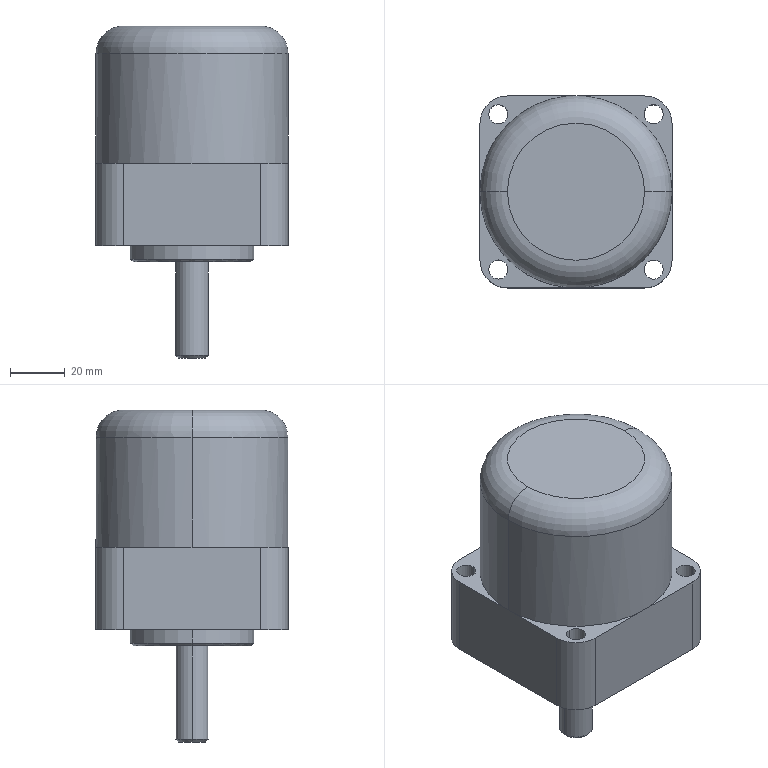Part | SolidWorks | features ICE 4, Chamfer 2, Fillet 2, CirPattern 1, Extrusion 1 | 1 solid | 36 faces | box 70 x 70 x 121 mm | volume 341225 mm3 | cylinder 18 | plane 12 | cone 4 | torus 2 | commonest cylinder face diameters 7 x8 20 x4 12 x2 45 x2 70 x2
STEP:
#1=CARTESIAN_POINT('',(-35.,0.,70.));
#2=VERTEX_POINT('',#1);
#3=CARTESIAN_POINT('',(35.,0.,70.));
#4=VERTEX_POINT('',#3);
#5=CARTESIAN_POINT('',(0.,0.,70.));
#6=DIRECTION('',(0.,0.,-1.));
#7=DIRECTION('',(1.,0.,0.));
#8=AXIS2_PLACEMENT_3D('',#5,#6,#7);
#9=CIRCLE('',#8,35.);
#10=EDGE_CURVE('',#2,#4,#9,.T.);
#11=ORIENTED_EDGE('',*,*,#10,.F.);
#12=CARTESIAN_POINT('',(-25.,0.,80.));
#13=VERTEX_POINT('',#12);
#14=CARTESIAN_POINT('',(-25.,0.,70.));
#15=DIRECTION('',(0.,1.,0.));
#16=DIRECTION('',(-1.,0.,0.));
#17=AXIS2_PLACEMENT_3D('',#14,#15,#16);
#18=CIRCLE('',#17,10.);
#19=EDGE_CURVE('',#2,#13,#18,.T.);
#20=ORIENTED_EDGE('',*,*,#19,.T.);
#21=CARTESIAN_POINT('',(25.,0.,80.));
#22=VERTEX_POINT('',#21);
#23=CARTESIAN_POINT('',(0.,0.,80.));
#24=DIRECTION('',(0.,0.,1.));
#25=DIRECTION('',(1.,0.,0.));
#26=AXIS2_PLACEMENT_3D('',#23,#24,#25);
#27=CIRCLE('',#26,25.);
#28=EDGE_CURVE('',#22,#13,#27,.T.);
#29=ORIENTED_EDGE('',*,*,#28,.F.);
#30=CARTESIAN_POINT('',(25.,0.,70.));
#31=DIRECTION('',(0.,-1.,0.));
#32=DIRECTION('',(0.,0.,-1.));
#33=AXIS2_PLACEMENT_3D('',#30,#31,#32);
#34=CIRCLE('',#33,10.);
#35=EDGE_CURVE('',#4,#22,#34,.T.);
#36=ORIENTED_EDGE('',*,*,#35,.F.);
#37=EDGE_LOOP('',(#11,#20,#29,#36));
#38=FACE_OUTER_BOUND('',#37,.T.);
#39=CARTESIAN_POINT('',(0.,0.,70.));
#40=DIRECTION('',(0.,0.,1.));
#41=DIRECTION('',(1.,0.,0.));
#42=AXIS2_PLACEMENT_3D('',#39,#40,#41);
#43=TOROIDAL_SURFACE('',#42,25.,10.);
#44=ADVANCED_FACE('',(#38),#43,.T.);
#45=ORIENTED_EDGE('',*,*,#10,.T.);
#46=CARTESIAN_POINT('',(35.,0.,30.));
#47=VERTEX_POINT('',#46);
#48=CARTESIAN_POINT('',(35.,0.,80.));
#49=DIRECTION('',(0.,0.,-1.));
#50=VECTOR('',#49,1000.);
#51=LINE('',#48,#50);
#52=EDGE_CURVE('',#4,#47,#51,.T.);
#53=ORIENTED_EDGE('',*,*,#52,.T.);
#54=CARTESIAN_POINT('',(0.,35.,30.));
#55=VERTEX_POINT('',#54);
#56=CARTESIAN_POINT('',(0.,0.,30.));
#57=DIRECTION('',(0.,0.,1.));
#58=DIRECTION('',(1.,0.,0.));
#59=AXIS2_PLACEMENT_3D('',#56,#57,#58);
#60=CIRCLE('',#59,35.);
#61=EDGE_CURVE('',#47,#55,#60,.T.);
#62=ORIENTED_EDGE('',*,*,#61,.T.);
#63=CARTESIAN_POINT('',(-35.,0.,30.));
#64=VERTEX_POINT('',#63);
#65=CARTESIAN_POINT('',(0.,0.,30.));
#66=DIRECTION('',(0.,0.,1.));
#67=DIRECTION('',(1.,0.,0.));
#68=AXIS2_PLACEMENT_3D('',#65,#66,#67);
#69=CIRCLE('',#68,35.);
#70=EDGE_CURVE('',#55,#64,#69,.T.);
#71=ORIENTED_EDGE('',*,*,#70,.T.);
#72=CARTESIAN_POINT('',(-35.,0.,80.));
#73=DIRECTION('',(0.,0.,-1.));
#74=VECTOR('',#73,1000.);
#75=LINE('',#72,#74);
#76=EDGE_CURVE('',#2,#64,#75,.T.);
#77=ORIENTED_EDGE('',*,*,#76,.F.);
#78=EDGE_LOOP('',(#45,#53,#62,#71,#77));
#79=FACE_OUTER_BOUND('',#78,.T.);
#80=CARTESIAN_POINT('',(0.,0.,80.));
#81=DIRECTION('',(0.,0.,-1.));
#82=DIRECTION('',(-1.,0.,0.));
#83=AXIS2_PLACEMENT_3D('',#80,#81,#82);
#84=CYLINDRICAL_SURFACE('',#83,35.);
#85=ADVANCED_FACE('',(#79),#84,.T.);
#86=CARTESIAN_POINT('',(28.284,31.784,0.));
#87=VERTEX_POINT('',#86);
#88=CARTESIAN_POINT('',(28.284,24.784,0.));
#89=VERTEX_POINT('',#88);
#90=CARTESIAN_POINT('',(28.284,28.284,0.));
#91=DIRECTION('',(0.,0.,1.));
#92=DIRECTION('',(0.,-1.,0.));
#93=AXIS2_PLACEMENT_3D('',#90,#91,#92);
#94=CIRCLE('',#93,3.5);
#95=EDGE_CURVE('',#87,#89,#94,.T.);
#96=ORIENTED_EDGE('',*,*,#95,.F.);
#97=CARTESIAN_POINT('',(28.284,31.784,30.));
#98=VERTEX_POINT('',#97);
#99=CARTESIAN_POINT('',(28.284,31.784,-30.));
#100=DIRECTION('',(0.,0.,1.));
#101=VECTOR('',#100,1000.);
#102=LINE('',#99,#101);
#103=EDGE_CURVE('',#87,#98,#102,.T.);
#104=ORIENTED_EDGE('',*,*,#103,.T.);
#105=CARTESIAN_POINT('',(28.284,24.784,30.));
#106=VERTEX_POINT('',#105);
#107=CARTESIAN_POINT('',(28.284,28.284,30.));
#108=DIRECTION('',(0.,0.,1.));
#109=DIRECTION('',(0.,-1.,0.));
#110=AXIS2_PLACEMENT_3D('',#107,#108,#109);
#111=CIRCLE('',#110,3.5);
#112=EDGE_CURVE('',#98,#106,#111,.T.);
#113=ORIENTED_EDGE('',*,*,#112,.T.);
#114=CARTESIAN_POINT('',(28.284,24.784,-30.));
#115=DIRECTION('',(0.,0.,1.));
#116=VECTOR('',#115,1000.);
#117=LINE('',#114,#116);
#118=EDGE_CURVE('',#89,#106,#117,.T.);
#119=ORIENTED_EDGE('',*,*,#118,.F.);
#120=EDGE_LOOP('',(#96,#104,#113,#119));
#121=FACE_OUTER_BOUND('',#120,.T.);
#122=CARTESIAN_POINT('',(28.284,28.284,-30.));
#123=DIRECTION('',(0.,0.,1.));
#124=DIRECTION('',(0.,-1.,0.));
#125=AXIS2_PLACEMENT_3D('',#122,#123,#124);
#126=CYLINDRICAL_SURFACE('',#125,3.5);
#127=ADVANCED_FACE('',(#121),#126,.F.);
#128=CARTESIAN_POINT('',(31.784,-28.284,0.));
#129=VERTEX_POINT('',#128);
#130=CARTESIAN_POINT('',(24.784,-28.284,0.));
#131=VERTEX_POINT('',#130);
#132=CARTESIAN_POINT('',(28.284,-28.284,0.));
#133=DIRECTION('',(0.,0.,1.));
#134=DIRECTION('',(-1.,0.,0.));
#135=AXIS2_PLACEMENT_3D('',#132,#133,#134);
#136=CIRCLE('',#135,3.5);
#137=EDGE_CURVE('',#129,#131,#136,.T.);
#138=ORIENTED_EDGE('',*,*,#137,.F.);
#139=CARTESIAN_POINT('',(31.784,-28.284,30.));
#140=VERTEX_POINT('',#139);
#141=CARTESIAN_POINT('',(31.784,-28.284,-30.));
#142=DIRECTION('',(0.,0.,1.));
#143=VECTOR('',#142,1000.);
#144=LINE('',#141,#143);
#145=EDGE_CURVE('',#129,#140,#144,.T.);
#146=ORIENTED_EDGE('',*,*,#145,.T.);
#147=CARTESIAN_POINT('',(24.784,-28.284,30.));
#148=VERTEX_POINT('',#147);
#149=CARTESIAN_POINT('',(28.284,-28.284,30.));
#150=DIRECTION('',(0.,0.,1.));
#151=DIRECTION('',(-1.,0.,0.));
#152=AXIS2_PLACEMENT_3D('',#149,#150,#151);
#153=CIRCLE('',#152,3.5);
#154=EDGE_CURVE('',#140,#148,#153,.T.);
#155=ORIENTED_EDGE('',*,*,#154,.T.);
#156=CARTESIAN_POINT('',(24.784,-28.284,-30.));
#157=DIRECTION('',(0.,0.,1.));
#158=VECTOR('',#157,1000.);
#159=LINE('',#156,#158);
#160=EDGE_CURVE('',#131,#148,#159,.T.);
#161=ORIENTED_EDGE('',*,*,#160,.F.);
#162=EDGE_LOOP('',(#138,#146,#155,#161));
#163=FACE_OUTER_BOUND('',#162,.T.);
#164=CARTESIAN_POINT('',(28.284,-28.284,-30.));
#165=DIRECTION('',(0.,0.,1.));
#166=DIRECTION('',(-1.,0.,0.));
#167=AXIS2_PLACEMENT_3D('',#164,#165,#166);
#168=CYLINDRICAL_SURFACE('',#167,3.5);
#169=ADVANCED_FACE('',(#163),#168,.F.);
#170=CARTESIAN_POINT('',(-28.284,-31.784,0.));
#171=VERTEX_POINT('',#170);
#172=CARTESIAN_POINT('',(-28.284,-24.784,0.));
#173=VERTEX_POINT('',#172);
#174=CARTESIAN_POINT('',(-28.284,-28.284,0.));
#175=DIRECTION('',(0.,0.,1.));
#176=DIRECTION('',(0.,1.,0.));
#177=AXIS2_PLACEMENT_3D('',#174,#175,#176);
#178=CIRCLE('',#177,3.5);
#179=EDGE_CURVE('',#171,#173,#178,.T.);
#180=ORIENTED_EDGE('',*,*,#179,.F.);
#181=CARTESIAN_POINT('',(-28.284,-31.784,30.));
#182=VERTEX_POINT('',#181);
#183=CARTESIAN_POINT('',(-28.284,-31.784,-30.));
#184=DIRECTION('',(0.,0.,1.));
#185=VECTOR('',#184,1000.);
#186=LINE('',#183,#185);
#187=EDGE_CURVE('',#171,#182,#186,.T.);
#188=ORIENTED_EDGE('',*,*,#187,.T.);
#189=CARTESIAN_POINT('',(-28.284,-24.784,30.));
#190=VERTEX_POINT('',#189);
#191=CARTESIAN_POINT('',(-28.284,-28.284,30.));
#192=DIRECTION('',(0.,0.,1.));
#193=DIRECTION('',(0.,1.,0.));
#194=AXIS2_PLACEMENT_3D('',#191,#192,#193);
#195=CIRCLE('',#194,3.5);
#196=EDGE_CURVE('',#182,#190,#195,.T.);
#197=ORIENTED_EDGE('',*,*,#196,.T.);
#198=CARTESIAN_POINT('',(-28.284,-24.784,-30.));
#199=DIRECTION('',(0.,0.,1.));
#200=VECTOR('',#199,1000.);
#201=LINE('',#198,#200);
#202=EDGE_CURVE('',#173,#190,#201,.T.);
#203=ORIENTED_EDGE('',*,*,#202,.F.);
#204=EDGE_LOOP('',(#180,#188,#197,#203));
#205=FACE_OUTER_BOUND('',#204,.T.);
#206=CARTESIAN_POINT('',(-28.284,-28.284,-30.));
#207=DIRECTION('',(0.,0.,1.));
#208=DIRECTION('',(0.,1.,0.));
#209=AXIS2_PLACEMENT_3D('',#206,#207,#208);
#210=CYLINDRICAL_SURFACE('',#209,3.5);
#211=ADVANCED_FACE('',(#205),#210,.F.);
#212=CARTESIAN_POINT('',(-21.5,0.,-6.));
#213=VERTEX_POINT('',#212);
#214=CARTESIAN_POINT('',(21.5,0.,-6.));
#215=VERTEX_POINT('',#214);
#216=CARTESIAN_POINT('',(0.,0.,-6.));
#217=DIRECTION('',(0.,0.,-1.));
#218=DIRECTION('',(-1.,0.,0.));
#219=AXIS2_PLACEMENT_3D('',#216,#217,#218);
#220=CIRCLE('',#219,21.5);
#221=EDGE_CURVE('',#213,#215,#220,.T.);
#222=ORIENTED_EDGE('',*,*,#221,.F.);
#223=CARTESIAN_POINT('',(-22.5,0.,-5.));
#224=VERTEX_POINT('',#223);
#225=CARTESIAN_POINT('',(-21.5,0.,-6.));
#226=DIRECTION('',(-0.7071,0.,0.7071));
#227=VECTOR('',#226,1000.);
#228=LINE('',#225,#227);
#229=EDGE_CURVE('',#213,#224,#228,.T.);
#230=ORIENTED_EDGE('',*,*,#229,.T.);
#231=CARTESIAN_POINT('',(22.5,0.,-5.));
#232=VERTEX_POINT('',#231);
#233=CARTESIAN_POINT('',(0.,0.,-5.));
#234=DIRECTION('',(0.,0.,1.));
#235=DIRECTION('',(-1.,0.,0.));
#236=AXIS2_PLACEMENT_3D('',#233,#234,#235);
#237=CIRCLE('',#236,22.5);
#238=EDGE_CURVE('',#232,#224,#237,.T.);
#239=ORIENTED_EDGE('',*,*,#238,.F.);
#240=CARTESIAN_POINT('',(21.5,0.,-6.));
#241=DIRECTION('',(0.7071,0.,0.7071));
#242=VECTOR('',#241,1000.);
#243=LINE('',#240,#242);
#244=EDGE_CURVE('',#215,#232,#243,.T.);
#245=ORIENTED_EDGE('',*,*,#244,.F.);
#246=EDGE_LOOP('',(#222,#230,#239,#245));
#247=FACE_OUTER_BOUND('',#246,.T.);
#248=CARTESIAN_POINT('',(0.,0.,-6.));
#249=DIRECTION('',(0.,0.,1.));
#250=DIRECTION('',(1.,0.,0.));
#251=AXIS2_PLACEMENT_3D('',#248,#249,#250);
#252=CONICAL_SURFACE('',#251,21.5,0.7854);
#253=ADVANCED_FACE('',(#247),#252,.T.);
#254=CARTESIAN_POINT('',(-5.,0.,-41.));
#255=VERTEX_POINT('',#254);
#256=CARTESIAN_POINT('',(5.,0.,-41.));
#257=VERTEX_POINT('',#256);
#258=CARTESIAN_POINT('',(0.,0.,-41.));
#259=DIRECTION('',(0.,0.,-1.));
#260=DIRECTION('',(-1.,0.,0.));
#261=AXIS2_PLACEMENT_3D('',#258,#259,#260);
#262=CIRCLE('',#261,5.);
#263=EDGE_CURVE('',#255,#257,#262,.T.);
#264=ORIENTED_EDGE('',*,*,#263,.F.);
#265=CARTESIAN_POINT('',(-6.,0.,-40.));
#266=VERTEX_POINT('',#265);
#267=CARTESIAN_POINT('',(-5.,0.,-41.));
#268=DIRECTION('',(-0.7071,0.,0.7071));
#269=VECTOR('',#268,1000.);
#270=LINE('',#267,#269);
#271=EDGE_CURVE('',#255,#266,#270,.T.);
#272=ORIENTED_EDGE('',*,*,#271,.T.);
#273=CARTESIAN_POINT('',(6.,0.,-40.));
#274=VERTEX_POINT('',#273);
#275=CARTESIAN_POINT('',(0.,0.,-40.));
#276=DIRECTION('',(0.,0.,1.));
#277=DIRECTION('',(-1.,0.,0.));
#278=AXIS2_PLACEMENT_3D('',#275,#276,#277);
#279=CIRCLE('',#278,6.);
#280=EDGE_CURVE('',#274,#266,#279,.T.);
#281=ORIENTED_EDGE('',*,*,#280,.F.);
#282=CARTESIAN_POINT('',(5.,0.,-41.));
#283=DIRECTION('',(0.7071,0.,0.7071));
#284=VECTOR('',#283,1000.);
#285=LINE('',#282,#284);
#286=EDGE_CURVE('',#257,#274,#285,.T.);
#287=ORIENTED_EDGE('',*,*,#286,.F.);
#288=EDGE_LOOP('',(#264,#272,#281,#287));
#289=FACE_OUTER_BOUND('',#288,.T.);
#290=CARTESIAN_POINT('',(0.,0.,-41.));
#291=DIRECTION('',(0.,0.,1.));
#292=DIRECTION('',(1.,0.,0.));
#293=AXIS2_PLACEMENT_3D('',#290,#291,#292);
#294=CONICAL_SURFACE('',#293,5.,0.7854);
#295=ADVANCED_FACE('',(#289),#294,.T.);
#296=ORIENTED_EDGE('',*,*,#280,.T.);
#297=CARTESIAN_POINT('',(-6.,0.,-6.));
#298=VERTEX_POINT('',#297);
#299=CARTESIAN_POINT('',(-6.,0.,-41.));
#300=DIRECTION('',(0.,0.,1.));
#301=VECTOR('',#300,1000.);
#302=LINE('',#299,#301);
#303=EDGE_CURVE('',#266,#298,#302,.T.);
#304=ORIENTED_EDGE('',*,*,#303,.T.);
#305=CARTESIAN_POINT('',(6.,0.,-6.));
#306=VERTEX_POINT('',#305);
#307=CARTESIAN_POINT('',(0.,0.,-6.));
#308=DIRECTION('',(0.,0.,-1.));
#309=DIRECTION('',(-1.,0.,0.));
#310=AXIS2_PLACEMENT_3D('',#307,#308,#309);
#311=CIRCLE('',#310,6.);
#312=EDGE_CURVE('',#298,#306,#311,.T.);
#313=ORIENTED_EDGE('',*,*,#312,.T.);
#314=CARTESIAN_POINT('',(6.,0.,-41.));
#315=DIRECTION('',(0.,0.,1.));
#316=VECTOR('',#315,1000.);
#317=LINE('',#314,#316);
#318=EDGE_CURVE('',#274,#306,#317,.T.);
#319=ORIENTED_EDGE('',*,*,#318,.F.);
#320=EDGE_LOOP('',(#296,#304,#313,#319));
#321=FACE_OUTER_BOUND('',#320,.T.);
#322=CARTESIAN_POINT('',(0.,0.,-41.));
#323=DIRECTION('',(0.,0.,1.));
#324=DIRECTION('',(1.,0.,0.));
#325=AXIS2_PLACEMENT_3D('',#322,#323,#324);
#326=CYLINDRICAL_SURFACE('',#325,6.);
#327=ADVANCED_FACE('',(#321),#326,.T.);
#328=ORIENTED_EDGE('',*,*,#238,.T.);
#329=CARTESIAN_POINT('',(-22.5,0.,0.));
#330=VERTEX_POINT('',#329);
#331=CARTESIAN_POINT('',(-22.5,0.,-6.));
#332=DIRECTION('',(0.,0.,1.));
#333=VECTOR('',#332,1000.);
#334=LINE('',#331,#333);
#335=EDGE_CURVE('',#224,#330,#334,.T.);
#336=ORIENTED_EDGE('',*,*,#335,.T.);
#337=CARTESIAN_POINT('',(22.5,0.,0.));
#338=VERTEX_POINT('',#337);
#339=CARTESIAN_POINT('',(0.,0.,0.));
#340=DIRECTION('',(0.,0.,-1.));
#341=DIRECTION('',(1.,0.,0.));
#342=AXIS2_PLACEMENT_3D('',#339,#340,#341);
#343=CIRCLE('',#342,22.5);
#344=EDGE_CURVE('',#330,#338,#343,.T.);
#345=ORIENTED_EDGE('',*,*,#344,.T.);
#346=CARTESIAN_POINT('',(22.5,0.,-6.));
#347=DIRECTION('',(0.,0.,1.));
#348=VECTOR('',#347,1000.);
#349=LINE('',#346,#348);
#350=EDGE_CURVE('',#232,#338,#349,.T.);
#351=ORIENTED_EDGE('',*,*,#350,.F.);
#352=EDGE_LOOP('',(#328,#336,#345,#351));
#353=FACE_OUTER_BOUND('',#352,.T.);
#354=CARTESIAN_POINT('',(0.,0.,-6.));
#355=DIRECTION('',(0.,0.,1.));
#356=DIRECTION('',(1.,0.,0.));
#357=AXIS2_PLACEMENT_3D('',#354,#355,#356);
#358=CYLINDRICAL_SURFACE('',#357,22.5);
#359=ADVANCED_FACE('',(#353),#358,.T.);
#360=CARTESIAN_POINT('',(-31.784,28.284,0.));
#361=VERTEX_POINT('',#360);
#362=CARTESIAN_POINT('',(-24.784,28.284,0.));
#363=VERTEX_POINT('',#362);
#364=CARTESIAN_POINT('',(-28.284,28.284,0.));
#365=DIRECTION('',(0.,0.,1.));
#366=DIRECTION('',(1.,0.,0.));
#367=AXIS2_PLACEMENT_3D('',#364,#365,#366);
#368=CIRCLE('',#367,3.5);
#369=EDGE_CURVE('',#361,#363,#368,.T.);
#370=ORIENTED_EDGE('',*,*,#369,.F.);
#371=CARTESIAN_POINT('',(-31.784,28.284,30.));
#372=VERTEX_POINT('',#371);
#373=CARTESIAN_POINT('',(-31.784,28.284,-30.));
#374=DIRECTION('',(0.,0.,1.));
#375=VECTOR('',#374,1000.);
#376=LINE('',#373,#375);
#377=EDGE_CURVE('',#361,#372,#376,.T.);
#378=ORIENTED_EDGE('',*,*,#377,.T.);
#379=CARTESIAN_POINT('',(-24.784,28.284,30.));
#380=VERTEX_POINT('',#379);
#381=CARTESIAN_POINT('',(-28.284,28.284,30.));
#382=DIRECTION('',(0.,0.,1.));
#383=DIRECTION('',(1.,0.,0.));
#384=AXIS2_PLACEMENT_3D('',#381,#382,#383);
#385=CIRCLE('',#384,3.5);
#386=EDGE_CURVE('',#372,#380,#385,.T.);
#387=ORIENTED_EDGE('',*,*,#386,.T.);
#388=CARTESIAN_POINT('',(-24.784,28.284,-30.));
#389=DIRECTION('',(0.,0.,1.));
#390=VECTOR('',#389,1000.);
#391=LINE('',#388,#390);
#392=EDGE_CURVE('',#363,#380,#391,.T.);
#393=ORIENTED_EDGE('',*,*,#392,.F.);
#394=EDGE_LOOP('',(#370,#378,#387,#393));
#395=FACE_OUTER_BOUND('',#394,.T.);
#396=CARTESIAN_POINT('',(-28.284,28.284,-30.));
#397=DIRECTION('',(0.,0.,1.));
#398=DIRECTION('',(1.,0.,0.));
#399=AXIS2_PLACEMENT_3D('',#396,#397,#398);
#400=CYLINDRICAL_SURFACE('',#399,3.5);
#401=ADVANCED_FACE('',(#395),#400,.F.);
#402=ORIENTED_EDGE('',*,*,#61,.F.);
#403=CARTESIAN_POINT('',(35.,25.,30.));
#404=VERTEX_POINT('',#403);
#405=CARTESIAN_POINT('',(35.,-35.,30.));
#406=DIRECTION('',(0.,1.,0.));
#407=VECTOR('',#406,1000.);
#408=LINE('',#405,#407);
#409=EDGE_CURVE('',#47,#404,#408,.T.);
#410=ORIENTED_EDGE('',*,*,#409,.T.);
#411=CARTESIAN_POINT('',(25.,35.,30.));
#412=VERTEX_POINT('',#411);
#413=CARTESIAN_POINT('',(25.,25.,30.));
#414=DIRECTION('',(0.,0.,1.));
#415=DIRECTION('',(1.,0.,0.));
#416=AXIS2_PLACEMENT_3D('',#413,#414,#415);
#417=CIRCLE('',#416,10.);
#418=EDGE_CURVE('',#404,#412,#417,.T.);
#419=ORIENTED_EDGE('',*,*,#418,.T.);
#420=CARTESIAN_POINT('',(35.,35.,30.));
#421=DIRECTION('',(-1.,0.,0.));
#422=VECTOR('',#421,1000.);
#423=LINE('',#420,#422);
#424=EDGE_CURVE('',#412,#55,#423,.T.);
#425=ORIENTED_EDGE('',*,*,#424,.T.);
#426=EDGE_LOOP('',(#402,#410,#419,#425));
#427=FACE_OUTER_BOUND('',#426,.T.);
#428=CARTESIAN_POINT('',(28.284,28.284,30.));
#429=DIRECTION('',(0.,0.,1.));
#430=DIRECTION('',(0.,-1.,0.));
#431=AXIS2_PLACEMENT_3D('',#428,#429,#430);
#432=CIRCLE('',#431,3.5);
#433=EDGE_CURVE('',#106,#98,#432,.T.);
#434=ORIENTED_EDGE('',*,*,#433,.F.);
#435=ORIENTED_EDGE('',*,*,#112,.F.);
#436=EDGE_LOOP('',(#434,#435));
#437=FACE_BOUND('',#436,.T.);
#438=CARTESIAN_POINT('',(0.,0.,30.));
#439=DIRECTION('',(0.,0.,1.));
#440=DIRECTION('',(1.,0.,0.));
#441=AXIS2_PLACEMENT_3D('',#438,#439,#440);
#442=PLANE('',#441);
#443=ADVANCED_FACE('',(#427,#437),#442,.T.);
#444=ORIENTED_EDGE('',*,*,#70,.F.);
#445=CARTESIAN_POINT('',(-25.,35.,30.));
#446=VERTEX_POINT('',#445);
#447=CARTESIAN_POINT('',(35.,35.,30.));
#448=DIRECTION('',(-1.,0.,0.));
#449=VECTOR('',#448,1000.);
#450=LINE('',#447,#449);
#451=EDGE_CURVE('',#55,#446,#450,.T.);
#452=ORIENTED_EDGE('',*,*,#451,.T.);
#453=CARTESIAN_POINT('',(-35.,25.,30.));
#454=VERTEX_POINT('',#453);
#455=CARTESIAN_POINT('',(-25.,25.,30.));
#456=DIRECTION('',(0.,0.,1.));
#457=DIRECTION('',(1.,0.,0.));
#458=AXIS2_PLACEMENT_3D('',#455,#456,#457);
#459=CIRCLE('',#458,10.);
#460=EDGE_CURVE('',#446,#454,#459,.T.);
#461=ORIENTED_EDGE('',*,*,#460,.T.);
#462=CARTESIAN_POINT('',(-35.,-35.,30.));
#463=DIRECTION('',(0.,-1.,0.));
#464=VECTOR('',#463,1000.);
#465=LINE('',#462,#464);
#466=EDGE_CURVE('',#454,#64,#465,.T.);
#467=ORIENTED_EDGE('',*,*,#466,.T.);
#468=EDGE_LOOP('',(#444,#452,#461,#467));
#469=FACE_OUTER_BOUND('',#468,.T.);
#470=CARTESIAN_POINT('',(-28.284,28.284,30.));
#471=DIRECTION('',(0.,0.,1.));
#472=DIRECTION('',(1.,0.,0.));
#473=AXIS2_PLACEMENT_3D('',#470,#471,#472);
#474=CIRCLE('',#473,3.5);
#475=EDGE_CURVE('',#380,#372,#474,.T.);
#476=ORIENTED_EDGE('',*,*,#475,.F.);
#477=ORIENTED_EDGE('',*,*,#386,.F.);
#478=EDGE_LOOP('',(#476,#477));
#479=FACE_BOUND('',#478,.T.);
#480=CARTESIAN_POINT('',(0.,0.,30.));
#481=DIRECTION('',(0.,0.,1.));
#482=DIRECTION('',(1.,0.,0.));
#483=AXIS2_PLACEMENT_3D('',#480,#481,#482);
#484=PLANE('',#483);
#485=ADVANCED_FACE('',(#469,#479),#484,.T.);
#486=CARTESIAN_POINT('',(0.,-35.,30.));
#487=VERTEX_POINT('',#486);
#488=CARTESIAN_POINT('',(0.,0.,30.));
#489=DIRECTION('',(0.,0.,1.));
#490=DIRECTION('',(1.,0.,0.));
#491=AXIS2_PLACEMENT_3D('',#488,#489,#490);
#492=CIRCLE('',#491,35.);
#493=EDGE_CURVE('',#64,#487,#492,.T.);
#494=ORIENTED_EDGE('',*,*,#493,.F.);
#495=CARTESIAN_POINT('',(-35.,-25.,30.));
#496=VERTEX_POINT('',#495);
#497=CARTESIAN_POINT('',(-35.,-35.,30.));
#498=DIRECTION('',(0.,-1.,0.));
#499=VECTOR('',#498,1000.);
#500=LINE('',#497,#499);
#501=EDGE_CURVE('',#64,#496,#500,.T.);
#502=ORIENTED_EDGE('',*,*,#501,.T.);
#503=CARTESIAN_POINT('',(-25.,-35.,30.));
#504=VERTEX_POINT('',#503);
#505=CARTESIAN_POINT('',(-25.,-25.,30.));
#506=DIRECTION('',(0.,0.,1.));
#507=DIRECTION('',(1.,0.,0.));
#508=AXIS2_PLACEMENT_3D('',#505,#506,#507);
#509=CIRCLE('',#508,10.);
#510=EDGE_CURVE('',#496,#504,#509,.T.);
#511=ORIENTED_EDGE('',*,*,#510,.T.);
#512=CARTESIAN_POINT('',(35.,-35.,30.));
#513=DIRECTION('',(1.,0.,0.));
#514=VECTOR('',#513,1000.);
#515=LINE('',#512,#514);
#516=EDGE_CURVE('',#504,#487,#515,.T.);
#517=ORIENTED_EDGE('',*,*,#516,.T.);
#518=EDGE_LOOP('',(#494,#502,#511,#517));
#519=FACE_OUTER_BOUND('',#518,.T.);
#520=CARTESIAN_POINT('',(-28.284,-28.284,30.));
#521=DIRECTION('',(0.,0.,1.));
#522=DIRECTION('',(0.,1.,0.));
#523=AXIS2_PLACEMENT_3D('',#520,#521,#522);
#524=CIRCLE('',#523,3.5);
#525=EDGE_CURVE('',#190,#182,#524,.T.);
#526=ORIENTED_EDGE('',*,*,#525,.F.);
#527=ORIENTED_EDGE('',*,*,#196,.F.);
#528=EDGE_LOOP('',(#526,#527));
#529=FACE_BOUND('',#528,.T.);
#530=CARTESIAN_POINT('',(0.,0.,30.));
#531=DIRECTION('',(0.,0.,1.));
#532=DIRECTION('',(1.,0.,0.));
#533=AXIS2_PLACEMENT_3D('',#530,#531,#532);
#534=PLANE('',#533);
#535=ADVANCED_FACE('',(#519,#529),#534,.T.);
#536=CARTESIAN_POINT('',(0.,0.,-6.));
#537=DIRECTION('',(0.,0.,-1.));
#538=DIRECTION('',(-1.,0.,0.));
#539=AXIS2_PLACEMENT_3D('',#536,#537,#538);
#540=CIRCLE('',#539,21.5);
#541=EDGE_CURVE('',#215,#213,#540,.T.);
#542=ORIENTED_EDGE('',*,*,#541,.T.);
#543=ORIENTED_EDGE('',*,*,#221,.T.);
#544=EDGE_LOOP('',(#542,#543));
#545=FACE_OUTER_BOUND('',#544,.T.);
#546=CARTESIAN_POINT('',(0.,0.,-6.));
#547=DIRECTION('',(0.,0.,-1.));
#548=DIRECTION('',(-1.,0.,0.));
#549=AXIS2_PLACEMENT_3D('',#546,#547,#548);
#550=CIRCLE('',#549,6.);
#551=EDGE_CURVE('',#306,#298,#550,.T.);
#552=ORIENTED_EDGE('',*,*,#551,.F.);
#553=ORIENTED_EDGE('',*,*,#312,.F.);
#554=EDGE_LOOP('',(#552,#553));
#555=FACE_BOUND('',#554,.T.);
#556=CARTESIAN_POINT('',(0.,0.,-6.));
#557=DIRECTION('',(0.,0.,-1.));
#558=DIRECTION('',(-1.,0.,0.));
#559=AXIS2_PLACEMENT_3D('',#556,#557,#558);
#560=PLANE('',#559);
#561=ADVANCED_FACE('',(#545,#555),#560,.T.);
#562=CARTESIAN_POINT('',(28.284,28.284,0.));
#563=DIRECTION('',(0.,0.,1.));
#564=DIRECTION('',(0.,-1.,0.));
#565=AXIS2_PLACEMENT_3D('',#562,#563,#564);
#566=CIRCLE('',#565,3.5);
#567=EDGE_CURVE('',#89,#87,#566,.T.);
#568=ORIENTED_EDGE('',*,*,#567,.T.);
#569=ORIENTED_EDGE('',*,*,#95,.T.);
#570=EDGE_LOOP('',(#568,#569));
#571=FACE_BOUND('',#570,.T.);
#572=CARTESIAN_POINT('',(28.284,-28.284,0.));
#573=DIRECTION('',(0.,0.,1.));
#574=DIRECTION('',(-1.,0.,0.));
#575=AXIS2_PLACEMENT_3D('',#572,#573,#574);
#576=CIRCLE('',#575,3.5);
#577=EDGE_CURVE('',#131,#129,#576,.T.);
#578=ORIENTED_EDGE('',*,*,#577,.T.);
#579=ORIENTED_EDGE('',*,*,#137,.T.);
#580=EDGE_LOOP('',(#578,#579));
#581=FACE_BOUND('',#580,.T.);
#582=CARTESIAN_POINT('',(-28.284,-28.284,0.));
#583=DIRECTION('',(0.,0.,1.));
#584=DIRECTION('',(0.,1.,0.));
#585=AXIS2_PLACEMENT_3D('',#582,#583,#584);
#586=CIRCLE('',#585,3.5);
#587=EDGE_CURVE('',#173,#171,#586,.T.);
#588=ORIENTED_EDGE('',*,*,#587,.T.);
#589=ORIENTED_EDGE('',*,*,#179,.T.);
#590=EDGE_LOOP('',(#588,#589));
#591=FACE_BOUND('',#590,.T.);
#592=CARTESIAN_POINT('',(35.,-25.,0.));
#593=VERTEX_POINT('',#592);
#594=CARTESIAN_POINT('',(35.,25.,0.));
#595=VERTEX_POINT('',#594);
#596=CARTESIAN_POINT('',(35.,-35.,0.));
#597=DIRECTION('',(0.,1.,0.));
#598=VECTOR('',#597,1000.);
#599=LINE('',#596,#598);
#600=EDGE_CURVE('',#593,#595,#599,.T.);
#601=ORIENTED_EDGE('',*,*,#600,.F.);
#602=CARTESIAN_POINT('',(25.,-35.,0.));
#603=VERTEX_POINT('',#602);
#604=CARTESIAN_POINT('',(25.,-25.,0.));
#605=DIRECTION('',(0.,0.,-1.));
#606=DIRECTION('',(1.,0.,0.));
#607=AXIS2_PLACEMENT_3D('',#604,#605,#606);
#608=CIRCLE('',#607,10.);
#609=EDGE_CURVE('',#593,#603,#608,.T.);
#610=ORIENTED_EDGE('',*,*,#609,.T.);
#611=CARTESIAN_POINT('',(-25.,-35.,0.));
#612=VERTEX_POINT('',#611);
#613=CARTESIAN_POINT('',(35.,-35.,0.));
#614=DIRECTION('',(1.,0.,0.));
#615=VECTOR('',#614,1000.);
#616=LINE('',#613,#615);
#617=EDGE_CURVE('',#612,#603,#616,.T.);
#618=ORIENTED_EDGE('',*,*,#617,.F.);
#619=CARTESIAN_POINT('',(-35.,-25.,0.));
#620=VERTEX_POINT('',#619);
#621=CARTESIAN_POINT('',(-25.,-25.,0.));
#622=DIRECTION('',(0.,0.,-1.));
#623=DIRECTION('',(1.,0.,0.));
#624=AXIS2_PLACEMENT_3D('',#621,#622,#623);
#625=CIRCLE('',#624,10.);
#626=EDGE_CURVE('',#612,#620,#625,.T.);
#627=ORIENTED_EDGE('',*,*,#626,.T.);
#628=CARTESIAN_POINT('',(-35.,25.,0.));
#629=VERTEX_POINT('',#628);
#630=CARTESIAN_POINT('',(-35.,-35.,0.));
#631=DIRECTION('',(0.,-1.,0.));
#632=VECTOR('',#631,1000.);
#633=LINE('',#630,#632);
#634=EDGE_CURVE('',#629,#620,#633,.T.);
#635=ORIENTED_EDGE('',*,*,#634,.F.);
#636=CARTESIAN_POINT('',(-25.,35.,0.));
#637=VERTEX_POINT('',#636);
#638=CARTESIAN_POINT('',(-25.,25.,0.));
#639=DIRECTION('',(0.,0.,-1.));
#640=DIRECTION('',(1.,0.,0.));
#641=AXIS2_PLACEMENT_3D('',#638,#639,#640);
#642=CIRCLE('',#641,10.);
#643=EDGE_CURVE('',#629,#637,#642,.T.);
#644=ORIENTED_EDGE('',*,*,#643,.T.);
#645=CARTESIAN_POINT('',(25.,35.,0.));
#646=VERTEX_POINT('',#645);
#647=CARTESIAN_POINT('',(35.,35.,0.));
#648=DIRECTION('',(-1.,0.,0.));
#649=VECTOR('',#648,1000.);
#650=LINE('',#647,#649);
#651=EDGE_CURVE('',#646,#637,#650,.T.);
#652=ORIENTED_EDGE('',*,*,#651,.F.);
#653=CARTESIAN_POINT('',(25.,25.,0.));
#654=DIRECTION('',(0.,0.,-1.));
#655=DIRECTION('',(1.,0.,0.));
#656=AXIS2_PLACEMENT_3D('',#653,#654,#655);
#657=CIRCLE('',#656,10.);
#658=EDGE_CURVE('',#646,#595,#657,.T.);
#659=ORIENTED_EDGE('',*,*,#658,.T.);
#660=EDGE_LOOP('',(#601,#610,#618,#627,#635,#644,#652,#659));
#661=FACE_OUTER_BOUND('',#660,.T.);
#662=CARTESIAN_POINT('',(-28.284,28.284,0.));
#663=DIRECTION('',(0.,0.,1.));
#664=DIRECTION('',(1.,0.,0.));
#665=AXIS2_PLACEMENT_3D('',#662,#663,#664);
#666=CIRCLE('',#665,3.5);
#667=EDGE_CURVE('',#363,#361,#666,.T.);
#668=ORIENTED_EDGE('',*,*,#667,.T.);
#669=ORIENTED_EDGE('',*,*,#369,.T.);
#670=EDGE_LOOP('',(#668,#669));
#671=FACE_BOUND('',#670,.T.);
#672=CARTESIAN_POINT('',(0.,0.,0.));
#673=DIRECTION('',(0.,0.,-1.));
#674=DIRECTION('',(1.,0.,0.));
#675=AXIS2_PLACEMENT_3D('',#672,#673,#674);
#676=CIRCLE('',#675,22.5);
#677=EDGE_CURVE('',#338,#330,#676,.T.);
#678=ORIENTED_EDGE('',*,*,#677,.F.);
#679=ORIENTED_EDGE('',*,*,#344,.F.);
#680=EDGE_LOOP('',(#678,#679));
#681=FACE_BOUND('',#680,.T.);
#682=CARTESIAN_POINT('',(0.,0.,0.));
#683=DIRECTION('',(0.,0.,1.));
#684=DIRECTION('',(1.,0.,0.));
#685=AXIS2_PLACEMENT_3D('',#682,#683,#684);
#686=PLANE('',#685);
#687=ADVANCED_FACE('',(#571,#581,#591,#661,#671,#681),#686,.F.);
#688=ORIENTED_EDGE('',*,*,#634,.T.);
#689=CARTESIAN_POINT('',(-35.,-25.,30.));
#690=DIRECTION('',(0.,0.,1.));
#691=VECTOR('',#690,1000.);
#692=LINE('',#689,#691);
#693=EDGE_CURVE('',#620,#496,#692,.T.);
#694=ORIENTED_EDGE('',*,*,#693,.T.);
#695=ORIENTED_EDGE('',*,*,#501,.F.);
#696=ORIENTED_EDGE('',*,*,#466,.F.);
#697=CARTESIAN_POINT('',(-35.,25.,30.));
#698=DIRECTION('',(0.,0.,-1.));
#699=VECTOR('',#698,1000.);
#700=LINE('',#697,#699);
#701=EDGE_CURVE('',#454,#629,#700,.T.);
#702=ORIENTED_EDGE('',*,*,#701,.T.);
#703=EDGE_LOOP('',(#688,#694,#695,#696,#702));
#704=FACE_OUTER_BOUND('',#703,.T.);
#705=CARTESIAN_POINT('',(-35.,-35.,30.));
#706=DIRECTION('',(1.,0.,0.));
#707=DIRECTION('',(0.,0.,-1.));
#708=AXIS2_PLACEMENT_3D('',#705,#706,#707);
#709=PLANE('',#708);
#710=ADVANCED_FACE('',(#704),#709,.F.);
#711=ORIENTED_EDGE('',*,*,#617,.T.);
#712=CARTESIAN_POINT('',(25.,-35.,30.));
#713=VERTEX_POINT('',#712);
#714=CARTESIAN_POINT('',(25.,-35.,30.));
#715=DIRECTION('',(0.,0.,1.));
#716=VECTOR('',#715,1000.);
#717=LINE('',#714,#716);
#718=EDGE_CURVE('',#603,#713,#717,.T.);
#719=ORIENTED_EDGE('',*,*,#718,.T.);
#720=CARTESIAN_POINT('',(35.,-35.,30.));
#721=DIRECTION('',(1.,0.,0.));
#722=VECTOR('',#721,1000.);
#723=LINE('',#720,#722);
#724=EDGE_CURVE('',#487,#713,#723,.T.);
#725=ORIENTED_EDGE('',*,*,#724,.F.);
#726=ORIENTED_EDGE('',*,*,#516,.F.);
#727=CARTESIAN_POINT('',(-25.,-35.,30.));
#728=DIRECTION('',(0.,0.,-1.));
#729=VECTOR('',#728,1000.);
#730=LINE('',#727,#729);
#731=EDGE_CURVE('',#504,#612,#730,.T.);
#732=ORIENTED_EDGE('',*,*,#731,.T.);
#733=EDGE_LOOP('',(#711,#719,#725,#726,#732));
#734=FACE_OUTER_BOUND('',#733,.T.);
#735=CARTESIAN_POINT('',(35.,-35.,30.));
#736=DIRECTION('',(0.,1.,0.));
#737=DIRECTION('',(-1.,0.,0.));
#738=AXIS2_PLACEMENT_3D('',#735,#736,#737);
#739=PLANE('',#738);
#740=ADVANCED_FACE('',(#734),#739,.F.);
#741=CARTESIAN_POINT('',(35.,-25.,30.));
#742=VERTEX_POINT('',#741);
#743=CARTESIAN_POINT('',(35.,-35.,30.));
#744=DIRECTION('',(0.,1.,0.));
#745=VECTOR('',#744,1000.);
#746=LINE('',#743,#745);
#747=EDGE_CURVE('',#742,#47,#746,.T.);
#748=ORIENTED_EDGE('',*,*,#747,.F.);
#749=CARTESIAN_POINT('',(35.,-25.,30.));
#750=DIRECTION('',(0.,0.,-1.));
#751=VECTOR('',#750,1000.);
#752=LINE('',#749,#751);
#753=EDGE_CURVE('',#742,#593,#752,.T.);
#754=ORIENTED_EDGE('',*,*,#753,.T.);
#755=ORIENTED_EDGE('',*,*,#600,.T.);
#756=CARTESIAN_POINT('',(35.,25.,30.));
#757=DIRECTION('',(0.,0.,1.));
#758=VECTOR('',#757,1000.);
#759=LINE('',#756,#758);
#760=EDGE_CURVE('',#595,#404,#759,.T.);
#761=ORIENTED_EDGE('',*,*,#760,.T.);
#762=ORIENTED_EDGE('',*,*,#409,.F.);
#763=EDGE_LOOP('',(#748,#754,#755,#761,#762));
#764=FACE_OUTER_BOUND('',#763,.T.);
#765=CARTESIAN_POINT('',(35.,-35.,30.));
#766=DIRECTION('',(-1.,0.,0.));
#767=DIRECTION('',(0.,0.,1.));
#768=AXIS2_PLACEMENT_3D('',#765,#766,#767);
#769=PLANE('',#768);
#770=ADVANCED_FACE('',(#764),#769,.F.);
#771=ORIENTED_EDGE('',*,*,#424,.F.);
#772=CARTESIAN_POINT('',(25.,35.,30.));
#773=DIRECTION('',(0.,0.,-1.));
#774=VECTOR('',#773,1000.);
#775=LINE('',#772,#774);
#776=EDGE_CURVE('',#412,#646,#775,.T.);
#777=ORIENTED_EDGE('',*,*,#776,.T.);
#778=ORIENTED_EDGE('',*,*,#651,.T.);
#779=CARTESIAN_POINT('',(-25.,35.,30.));
#780=DIRECTION('',(0.,0.,1.));
#781=VECTOR('',#780,1000.);
#782=LINE('',#779,#781);
#783=EDGE_CURVE('',#637,#446,#782,.T.);
#784=ORIENTED_EDGE('',*,*,#783,.T.);
#785=ORIENTED_EDGE('',*,*,#451,.F.);
#786=EDGE_LOOP('',(#771,#777,#778,#784,#785));
#787=FACE_OUTER_BOUND('',#786,.T.);
#788=CARTESIAN_POINT('',(35.,35.,30.));
#789=DIRECTION('',(0.,-1.,0.));
#790=DIRECTION('',(1.,0.,0.));
#791=AXIS2_PLACEMENT_3D('',#788,#789,#790);
#792=PLANE('',#791);
#793=ADVANCED_FACE('',(#787),#792,.F.);
#794=CARTESIAN_POINT('',(0.,0.,30.));
#795=DIRECTION('',(0.,0.,1.));
#796=DIRECTION('',(1.,0.,0.));
#797=AXIS2_PLACEMENT_3D('',#794,#795,#796);
#798=CIRCLE('',#797,35.);
#799=EDGE_CURVE('',#487,#47,#798,.T.);
#800=ORIENTED_EDGE('',*,*,#799,.F.);
#801=ORIENTED_EDGE('',*,*,#724,.T.);
#802=CARTESIAN_POINT('',(25.,-25.,30.));
#803=DIRECTION('',(0.,0.,1.));
#804=DIRECTION('',(1.,0.,0.));
#805=AXIS2_PLACEMENT_3D('',#802,#803,#804);
#806=CIRCLE('',#805,10.);
#807=EDGE_CURVE('',#713,#742,#806,.T.);
#808=ORIENTED_EDGE('',*,*,#807,.T.);
#809=ORIENTED_EDGE('',*,*,#747,.T.);
#810=EDGE_LOOP('',(#800,#801,#808,#809));
#811=FACE_OUTER_BOUND('',#810,.T.);
#812=CARTESIAN_POINT('',(28.284,-28.284,30.));
#813=DIRECTION('',(0.,0.,1.));
#814=DIRECTION('',(-1.,0.,0.));
#815=AXIS2_PLACEMENT_3D('',#812,#813,#814);
#816=CIRCLE('',#815,3.5);
#817=EDGE_CURVE('',#148,#140,#816,.T.);
#818=ORIENTED_EDGE('',*,*,#817,.F.);
#819=ORIENTED_EDGE('',*,*,#154,.F.);
#820=EDGE_LOOP('',(#818,#819));
#821=FACE_BOUND('',#820,.T.);
#822=CARTESIAN_POINT('',(0.,0.,30.));
#823=DIRECTION('',(0.,0.,1.));
#824=DIRECTION('',(1.,0.,0.));
#825=AXIS2_PLACEMENT_3D('',#822,#823,#824);
#826=PLANE('',#825);
#827=ADVANCED_FACE('',(#811,#821),#826,.T.);
#828=ORIENTED_EDGE('',*,*,#807,.F.);
#829=ORIENTED_EDGE('',*,*,#718,.F.);
#830=ORIENTED_EDGE('',*,*,#609,.F.);
#831=ORIENTED_EDGE('',*,*,#753,.F.);
#832=EDGE_LOOP('',(#828,#829,#830,#831));
#833=FACE_OUTER_BOUND('',#832,.T.);
#834=CARTESIAN_POINT('',(25.,-25.,30.));
#835=DIRECTION('',(0.,0.,-1.));
#836=DIRECTION('',(-1.,0.,0.));
#837=AXIS2_PLACEMENT_3D('',#834,#835,#836);
#838=CYLINDRICAL_SURFACE('',#837,10.);
#839=ADVANCED_FACE('',(#833),#838,.T.);
#840=ORIENTED_EDGE('',*,*,#510,.F.);
#841=ORIENTED_EDGE('',*,*,#693,.F.);
#842=ORIENTED_EDGE('',*,*,#626,.F.);
#843=ORIENTED_EDGE('',*,*,#731,.F.);
#844=EDGE_LOOP('',(#840,#841,#842,#843));
#845=FACE_OUTER_BOUND('',#844,.T.);
#846=CARTESIAN_POINT('',(-25.,-25.,30.));
#847=DIRECTION('',(0.,0.,-1.));
#848=DIRECTION('',(-1.,0.,0.));
#849=AXIS2_PLACEMENT_3D('',#846,#847,#848);
#850=CYLINDRICAL_SURFACE('',#849,10.);
#851=ADVANCED_FACE('',(#845),#850,.T.);
#852=ORIENTED_EDGE('',*,*,#418,.F.);
#853=ORIENTED_EDGE('',*,*,#760,.F.);
#854=ORIENTED_EDGE('',*,*,#658,.F.);
#855=ORIENTED_EDGE('',*,*,#776,.F.);
#856=EDGE_LOOP('',(#852,#853,#854,#855));
#857=FACE_OUTER_BOUND('',#856,.T.);
#858=CARTESIAN_POINT('',(25.,25.,30.));
#859=DIRECTION('',(0.,0.,-1.));
#860=DIRECTION('',(-1.,0.,0.));
#861=AXIS2_PLACEMENT_3D('',#858,#859,#860);
#862=CYLINDRICAL_SURFACE('',#861,10.);
#863=ADVANCED_FACE('',(#857),#862,.T.);
#864=ORIENTED_EDGE('',*,*,#460,.F.);
#865=ORIENTED_EDGE('',*,*,#783,.F.);
#866=ORIENTED_EDGE('',*,*,#643,.F.);
#867=ORIENTED_EDGE('',*,*,#701,.F.);
#868=EDGE_LOOP('',(#864,#865,#866,#867));
#869=FACE_OUTER_BOUND('',#868,.T.);
#870=CARTESIAN_POINT('',(-25.,25.,30.));
#871=DIRECTION('',(0.,0.,-1.));
#872=DIRECTION('',(-1.,0.,0.));
#873=AXIS2_PLACEMENT_3D('',#870,#871,#872);
#874=CYLINDRICAL_SURFACE('',#873,10.);
#875=ADVANCED_FACE('',(#869),#874,.T.);
#876=ORIENTED_EDGE('',*,*,#377,.F.);
#877=ORIENTED_EDGE('',*,*,#667,.F.);
#878=ORIENTED_EDGE('',*,*,#392,.T.);
#879=ORIENTED_EDGE('',*,*,#475,.T.);
#880=EDGE_LOOP('',(#876,#877,#878,#879));
#881=FACE_OUTER_BOUND('',#880,.T.);
#882=CARTESIAN_POINT('',(-28.284,28.284,-30.));
#883=DIRECTION('',(0.,0.,1.));
#884=DIRECTION('',(1.,0.,0.));
#885=AXIS2_PLACEMENT_3D('',#882,#883,#884);
#886=CYLINDRICAL_SURFACE('',#885,3.5);
#887=ADVANCED_FACE('',(#881),#886,.F.);
#888=ORIENTED_EDGE('',*,*,#335,.F.);
#889=CARTESIAN_POINT('',(0.,0.,-5.));
#890=DIRECTION('',(0.,0.,1.));
#891=DIRECTION('',(-1.,0.,0.));
#892=AXIS2_PLACEMENT_3D('',#889,#890,#891);
#893=CIRCLE('',#892,22.5);
#894=EDGE_CURVE('',#224,#232,#893,.T.);
#895=ORIENTED_EDGE('',*,*,#894,.T.);
#896=ORIENTED_EDGE('',*,*,#350,.T.);
#897=ORIENTED_EDGE('',*,*,#677,.T.);
#898=EDGE_LOOP('',(#888,#895,#896,#897));
#899=FACE_OUTER_BOUND('',#898,.T.);
#900=CARTESIAN_POINT('',(0.,0.,-6.));
#901=DIRECTION('',(0.,0.,1.));
#902=DIRECTION('',(1.,0.,0.));
#903=AXIS2_PLACEMENT_3D('',#900,#901,#902);
#904=CYLINDRICAL_SURFACE('',#903,22.5);
#905=ADVANCED_FACE('',(#899),#904,.T.);
#906=ORIENTED_EDGE('',*,*,#303,.F.);
#907=CARTESIAN_POINT('',(0.,0.,-40.));
#908=DIRECTION('',(0.,0.,1.));
#909=DIRECTION('',(-1.,0.,0.));
#910=AXIS2_PLACEMENT_3D('',#907,#908,#909);
#911=CIRCLE('',#910,6.);
#912=EDGE_CURVE('',#266,#274,#911,.T.);
#913=ORIENTED_EDGE('',*,*,#912,.T.);
#914=ORIENTED_EDGE('',*,*,#318,.T.);
#915=ORIENTED_EDGE('',*,*,#551,.T.);
#916=EDGE_LOOP('',(#906,#913,#914,#915));
#917=FACE_OUTER_BOUND('',#916,.T.);
#918=CARTESIAN_POINT('',(0.,0.,-41.));
#919=DIRECTION('',(0.,0.,1.));
#920=DIRECTION('',(1.,0.,0.));
#921=AXIS2_PLACEMENT_3D('',#918,#919,#920);
#922=CYLINDRICAL_SURFACE('',#921,6.);
#923=ADVANCED_FACE('',(#917),#922,.T.);
#924=CARTESIAN_POINT('',(0.,0.,-41.));
#925=DIRECTION('',(0.,0.,-1.));
#926=DIRECTION('',(-1.,0.,0.));
#927=AXIS2_PLACEMENT_3D('',#924,#925,#926);
#928=CIRCLE('',#927,5.);
#929=EDGE_CURVE('',#257,#255,#928,.T.);
#930=ORIENTED_EDGE('',*,*,#929,.T.);
#931=ORIENTED_EDGE('',*,*,#263,.T.);
#932=EDGE_LOOP('',(#930,#931));
#933=FACE_OUTER_BOUND('',#932,.T.);
#934=CARTESIAN_POINT('',(0.,0.,-41.));
#935=DIRECTION('',(0.,0.,-1.));
#936=DIRECTION('',(-1.,0.,0.));
#937=AXIS2_PLACEMENT_3D('',#934,#935,#936);
#938=PLANE('',#937);
#939=ADVANCED_FACE('',(#933),#938,.T.);
#940=ORIENTED_EDGE('',*,*,#271,.F.);
#941=ORIENTED_EDGE('',*,*,#929,.F.);
#942=ORIENTED_EDGE('',*,*,#286,.T.);
#943=ORIENTED_EDGE('',*,*,#912,.F.);
#944=EDGE_LOOP('',(#940,#941,#942,#943));
#945=FACE_OUTER_BOUND('',#944,.T.);
#946=CARTESIAN_POINT('',(0.,0.,-41.));
#947=DIRECTION('',(0.,0.,1.));
#948=DIRECTION('',(1.,0.,0.));
#949=AXIS2_PLACEMENT_3D('',#946,#947,#948);
#950=CONICAL_SURFACE('',#949,5.,0.7854);
#951=ADVANCED_FACE('',(#945),#950,.T.);
#952=ORIENTED_EDGE('',*,*,#229,.F.);
#953=ORIENTED_EDGE('',*,*,#541,.F.);
#954=ORIENTED_EDGE('',*,*,#244,.T.);
#955=ORIENTED_EDGE('',*,*,#894,.F.);
#956=EDGE_LOOP('',(#952,#953,#954,#955));
#957=FACE_OUTER_BOUND('',#956,.T.);
#958=CARTESIAN_POINT('',(0.,0.,-6.));
#959=DIRECTION('',(0.,0.,1.));
#960=DIRECTION('',(1.,0.,0.));
#961=AXIS2_PLACEMENT_3D('',#958,#959,#960);
#962=CONICAL_SURFACE('',#961,21.5,0.7854);
#963=ADVANCED_FACE('',(#957),#962,.T.);
#964=ORIENTED_EDGE('',*,*,#187,.F.);
#965=ORIENTED_EDGE('',*,*,#587,.F.);
#966=ORIENTED_EDGE('',*,*,#202,.T.);
#967=ORIENTED_EDGE('',*,*,#525,.T.);
#968=EDGE_LOOP('',(#964,#965,#966,#967));
#969=FACE_OUTER_BOUND('',#968,.T.);
#970=CARTESIAN_POINT('',(-28.284,-28.284,-30.));
#971=DIRECTION('',(0.,0.,1.));
#972=DIRECTION('',(0.,1.,0.));
#973=AXIS2_PLACEMENT_3D('',#970,#971,#972);
#974=CYLINDRICAL_SURFACE('',#973,3.5);
#975=ADVANCED_FACE('',(#969),#974,.F.);
#976=ORIENTED_EDGE('',*,*,#145,.F.);
#977=ORIENTED_EDGE('',*,*,#577,.F.);
#978=ORIENTED_EDGE('',*,*,#160,.T.);
#979=ORIENTED_EDGE('',*,*,#817,.T.);
#980=EDGE_LOOP('',(#976,#977,#978,#979));
#981=FACE_OUTER_BOUND('',#980,.T.);
#982=CARTESIAN_POINT('',(28.284,-28.284,-30.));
#983=DIRECTION('',(0.,0.,1.));
#984=DIRECTION('',(-1.,0.,0.));
#985=AXIS2_PLACEMENT_3D('',#982,#983,#984);
#986=CYLINDRICAL_SURFACE('',#985,3.5);
#987=ADVANCED_FACE('',(#981),#986,.F.);
#988=ORIENTED_EDGE('',*,*,#103,.F.);
#989=ORIENTED_EDGE('',*,*,#567,.F.);
#990=ORIENTED_EDGE('',*,*,#118,.T.);
#991=ORIENTED_EDGE('',*,*,#433,.T.);
#992=EDGE_LOOP('',(#988,#989,#990,#991));
#993=FACE_OUTER_BOUND('',#992,.T.);
#994=CARTESIAN_POINT('',(28.284,28.284,-30.));
#995=DIRECTION('',(0.,0.,1.));
#996=DIRECTION('',(0.,-1.,0.));
#997=AXIS2_PLACEMENT_3D('',#994,#995,#996);
#998=CYLINDRICAL_SURFACE('',#997,3.5);
#999=ADVANCED_FACE('',(#993),#998,.F.);
#1000=ORIENTED_EDGE('',*,*,#52,.F.);
#1001=CARTESIAN_POINT('',(0.,0.,70.));
#1002=DIRECTION('',(0.,0.,-1.));
#1003=DIRECTION('',(1.,0.,0.));
#1004=AXIS2_PLACEMENT_3D('',#1001,#1002,#1003);
#1005=CIRCLE('',#1004,35.);
#1006=EDGE_CURVE('',#4,#2,#1005,.T.);
#1007=ORIENTED_EDGE('',*,*,#1006,.T.);
#1008=ORIENTED_EDGE('',*,*,#76,.T.);
#1009=ORIENTED_EDGE('',*,*,#493,.T.);
#1010=ORIENTED_EDGE('',*,*,#799,.T.);
#1011=EDGE_LOOP('',(#1000,#1007,#1008,#1009,#1010));
#1012=FACE_OUTER_BOUND('',#1011,.T.);
#1013=CARTESIAN_POINT('',(0.,0.,80.));
#1014=DIRECTION('',(0.,0.,-1.));
#1015=DIRECTION('',(-1.,0.,0.));
#1016=AXIS2_PLACEMENT_3D('',#1013,#1014,#1015);
#1017=CYLINDRICAL_SURFACE('',#1016,35.);
#1018=ADVANCED_FACE('',(#1012),#1017,.T.);
#1019=ORIENTED_EDGE('',*,*,#28,.T.);
#1020=CARTESIAN_POINT('',(0.,0.,80.));
#1021=DIRECTION('',(0.,0.,1.));
#1022=DIRECTION('',(1.,0.,0.));
#1023=AXIS2_PLACEMENT_3D('',#1020,#1021,#1022);
#1024=CIRCLE('',#1023,25.);
#1025=EDGE_CURVE('',#13,#22,#1024,.T.);
#1026=ORIENTED_EDGE('',*,*,#1025,.T.);
#1027=EDGE_LOOP('',(#1019,#1026));
#1028=FACE_OUTER_BOUND('',#1027,.T.);
#1029=CARTESIAN_POINT('',(0.,0.,80.));
#1030=DIRECTION('',(0.,0.,1.));
#1031=DIRECTION('',(1.,0.,0.));
#1032=AXIS2_PLACEMENT_3D('',#1029,#1030,#1031);
#1033=PLANE('',#1032);
#1034=ADVANCED_FACE('',(#1028),#1033,.T.);
#1035=ORIENTED_EDGE('',*,*,#19,.F.);
#1036=ORIENTED_EDGE('',*,*,#1006,.F.);
#1037=ORIENTED_EDGE('',*,*,#35,.T.);
#1038=ORIENTED_EDGE('',*,*,#1025,.F.);
#1039=EDGE_LOOP('',(#1035,#1036,#1037,#1038));
#1040=FACE_OUTER_BOUND('',#1039,.T.);
#1041=CARTESIAN_POINT('',(0.,0.,70.));
#1042=DIRECTION('',(0.,0.,1.));
#1043=DIRECTION('',(1.,0.,0.));
#1044=AXIS2_PLACEMENT_3D('',#1041,#1042,#1043);
#1045=TOROIDAL_SURFACE('',#1044,25.,10.);
#1046=ADVANCED_FACE('',(#1040),#1045,.T.);
#1047=CLOSED_SHELL('',(#44,#85,#127,#169,#211,#253,#295,#327,#359,#401,#443,#485,#535,#561,#687,#710,#740,#770,#793,#827,#839,#851,#863,#875,#887,#905,#923,#939,#951,#963,#975,#987,#999,#1018,#1034,#1046));
#1048=MANIFOLD_SOLID_BREP('',#1047);
#1049=CARTESIAN_POINT('',(0.,0.,0.));
#1050=DIRECTION('',(0.,0.,1.));
#1051=DIRECTION('',(1.,0.,0.));
#1052=AXIS2_PLACEMENT_3D('',#1049,#1050,#1051);
#1053=(LENGTH_UNIT()NAMED_UNIT(*)SI_UNIT(.MILLI.,.METRE.));
#1054=UNCERTAINTY_MEASURE_WITH_UNIT(LENGTH_MEASURE(0.00001),#1053,'','');
#1055=(NAMED_UNIT(*)PLANE_ANGLE_UNIT()SI_UNIT($,.RADIAN.));
#1056=(NAMED_UNIT(*)SI_UNIT($,.STERADIAN.)SOLID_ANGLE_UNIT());
#1057=(GEOMETRIC_REPRESENTATION_CONTEXT(3)GLOBAL_UNCERTAINTY_ASSIGNED_CONTEXT((#1054))GLOBAL_UNIT_ASSIGNED_CONTEXT((#1053,#1055,#1056))REPRESENTATION_CONTEXT('',''));
#1058=ADVANCED_BREP_SHAPE_REPRESENTATION('',(#1048,#1052),#1057);